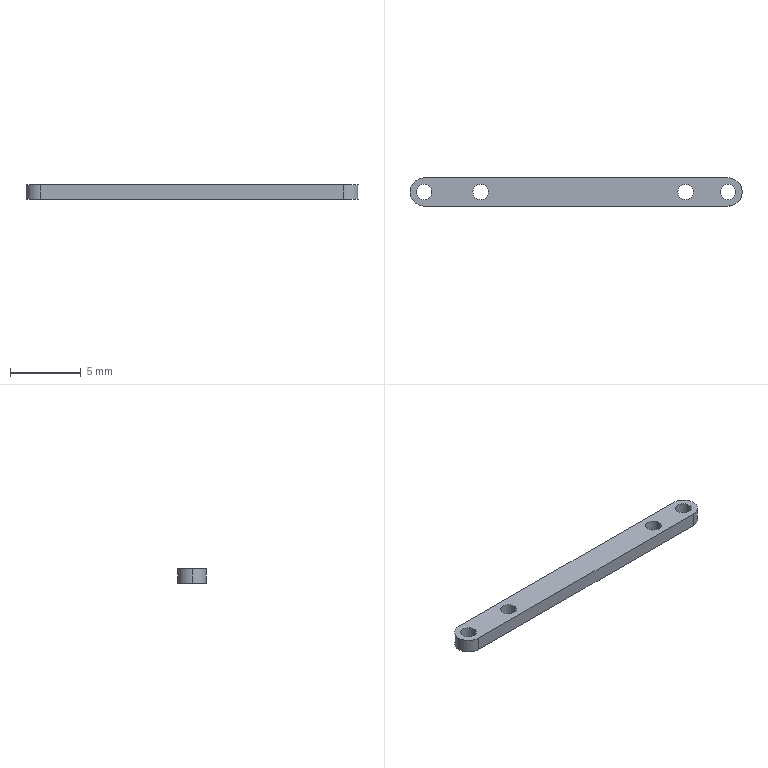Part | SolidWorks | features Extrusion 1, ICE 1 | 1 solid | 15 faces | box 23.5 x 2 x 1 mm | volume 42.34 mm3 | cylinder 11 | plane 4 | commonest cylinder face diameters 1.1 x8 2 x3
STEP:
#1=CARTESIAN_POINT('',(7.2,0.,0.5));
#2=VERTEX_POINT('',#1);
#3=CARTESIAN_POINT('',(8.3,0.,0.5));
#4=VERTEX_POINT('',#3);
#5=CARTESIAN_POINT('',(7.75,0.,0.5));
#6=DIRECTION('',(0.,0.,1.));
#7=DIRECTION('',(1.,0.,0.));
#8=AXIS2_PLACEMENT_3D('',#5,#6,#7);
#9=CIRCLE('',#8,0.55);
#10=EDGE_CURVE('',#2,#4,#9,.T.);
#11=ORIENTED_EDGE('',*,*,#10,.T.);
#12=CARTESIAN_POINT('',(8.3,0.,-0.5));
#13=VERTEX_POINT('',#12);
#14=CARTESIAN_POINT('',(8.3,0.,0.5));
#15=DIRECTION('',(0.,0.,-1.));
#16=VECTOR('',#15,1000.);
#17=LINE('',#14,#16);
#18=EDGE_CURVE('',#4,#13,#17,.T.);
#19=ORIENTED_EDGE('',*,*,#18,.T.);
#20=CARTESIAN_POINT('',(7.2,0.,-0.5));
#21=VERTEX_POINT('',#20);
#22=CARTESIAN_POINT('',(7.75,0.,-0.5));
#23=DIRECTION('',(0.,0.,1.));
#24=DIRECTION('',(1.,0.,0.));
#25=AXIS2_PLACEMENT_3D('',#22,#23,#24);
#26=CIRCLE('',#25,0.55);
#27=EDGE_CURVE('',#21,#13,#26,.T.);
#28=ORIENTED_EDGE('',*,*,#27,.F.);
#29=CARTESIAN_POINT('',(7.2,0.,0.5));
#30=DIRECTION('',(0.,0.,-1.));
#31=VECTOR('',#30,1000.);
#32=LINE('',#29,#31);
#33=EDGE_CURVE('',#2,#21,#32,.T.);
#34=ORIENTED_EDGE('',*,*,#33,.F.);
#35=EDGE_LOOP('',(#11,#19,#28,#34));
#36=FACE_OUTER_BOUND('',#35,.T.);
#37=CARTESIAN_POINT('',(7.75,0.,0.5));
#38=DIRECTION('',(0.,0.,-1.));
#39=DIRECTION('',(-1.,0.,0.));
#40=AXIS2_PLACEMENT_3D('',#37,#38,#39);
#41=CYLINDRICAL_SURFACE('',#40,0.55);
#42=ADVANCED_FACE('',(#36),#41,.F.);
#43=CARTESIAN_POINT('',(-7.3,0.,0.5));
#44=VERTEX_POINT('',#43);
#45=CARTESIAN_POINT('',(-6.2,0.,0.5));
#46=VERTEX_POINT('',#45);
#47=CARTESIAN_POINT('',(-6.75,0.,0.5));
#48=DIRECTION('',(0.,0.,1.));
#49=DIRECTION('',(1.,0.,0.));
#50=AXIS2_PLACEMENT_3D('',#47,#48,#49);
#51=CIRCLE('',#50,0.55);
#52=EDGE_CURVE('',#44,#46,#51,.T.);
#53=ORIENTED_EDGE('',*,*,#52,.T.);
#54=CARTESIAN_POINT('',(-6.2,0.,-0.5));
#55=VERTEX_POINT('',#54);
#56=CARTESIAN_POINT('',(-6.2,0.,0.5));
#57=DIRECTION('',(0.,0.,-1.));
#58=VECTOR('',#57,1000.);
#59=LINE('',#56,#58);
#60=EDGE_CURVE('',#46,#55,#59,.T.);
#61=ORIENTED_EDGE('',*,*,#60,.T.);
#62=CARTESIAN_POINT('',(-7.3,0.,-0.5));
#63=VERTEX_POINT('',#62);
#64=CARTESIAN_POINT('',(-6.75,0.,-0.5));
#65=DIRECTION('',(0.,0.,1.));
#66=DIRECTION('',(1.,0.,0.));
#67=AXIS2_PLACEMENT_3D('',#64,#65,#66);
#68=CIRCLE('',#67,0.55);
#69=EDGE_CURVE('',#63,#55,#68,.T.);
#70=ORIENTED_EDGE('',*,*,#69,.F.);
#71=CARTESIAN_POINT('',(-7.3,0.,0.5));
#72=DIRECTION('',(0.,0.,-1.));
#73=VECTOR('',#72,1000.);
#74=LINE('',#71,#73);
#75=EDGE_CURVE('',#44,#63,#74,.T.);
#76=ORIENTED_EDGE('',*,*,#75,.F.);
#77=EDGE_LOOP('',(#53,#61,#70,#76));
#78=FACE_OUTER_BOUND('',#77,.T.);
#79=CARTESIAN_POINT('',(-6.75,0.,0.5));
#80=DIRECTION('',(0.,0.,-1.));
#81=DIRECTION('',(-1.,0.,0.));
#82=AXIS2_PLACEMENT_3D('',#79,#80,#81);
#83=CYLINDRICAL_SURFACE('',#82,0.55);
#84=ADVANCED_FACE('',(#78),#83,.F.);
#85=CARTESIAN_POINT('',(10.2,0.,0.5));
#86=VERTEX_POINT('',#85);
#87=CARTESIAN_POINT('',(11.3,0.,0.5));
#88=VERTEX_POINT('',#87);
#89=CARTESIAN_POINT('',(10.75,0.,0.5));
#90=DIRECTION('',(0.,0.,1.));
#91=DIRECTION('',(1.,0.,0.));
#92=AXIS2_PLACEMENT_3D('',#89,#90,#91);
#93=CIRCLE('',#92,0.55);
#94=EDGE_CURVE('',#86,#88,#93,.T.);
#95=ORIENTED_EDGE('',*,*,#94,.T.);
#96=CARTESIAN_POINT('',(11.3,0.,-0.5));
#97=VERTEX_POINT('',#96);
#98=CARTESIAN_POINT('',(11.3,0.,0.5));
#99=DIRECTION('',(0.,0.,-1.));
#100=VECTOR('',#99,1000.);
#101=LINE('',#98,#100);
#102=EDGE_CURVE('',#88,#97,#101,.T.);
#103=ORIENTED_EDGE('',*,*,#102,.T.);
#104=CARTESIAN_POINT('',(10.2,0.,-0.5));
#105=VERTEX_POINT('',#104);
#106=CARTESIAN_POINT('',(10.75,0.,-0.5));
#107=DIRECTION('',(0.,0.,1.));
#108=DIRECTION('',(1.,0.,0.));
#109=AXIS2_PLACEMENT_3D('',#106,#107,#108);
#110=CIRCLE('',#109,0.55);
#111=EDGE_CURVE('',#105,#97,#110,.T.);
#112=ORIENTED_EDGE('',*,*,#111,.F.);
#113=CARTESIAN_POINT('',(10.2,0.,0.5));
#114=DIRECTION('',(0.,0.,-1.));
#115=VECTOR('',#114,1000.);
#116=LINE('',#113,#115);
#117=EDGE_CURVE('',#86,#105,#116,.T.);
#118=ORIENTED_EDGE('',*,*,#117,.F.);
#119=EDGE_LOOP('',(#95,#103,#112,#118));
#120=FACE_OUTER_BOUND('',#119,.T.);
#121=CARTESIAN_POINT('',(10.75,0.,0.5));
#122=DIRECTION('',(0.,0.,-1.));
#123=DIRECTION('',(-1.,0.,0.));
#124=AXIS2_PLACEMENT_3D('',#121,#122,#123);
#125=CYLINDRICAL_SURFACE('',#124,0.55);
#126=ADVANCED_FACE('',(#120),#125,.F.);
#127=CARTESIAN_POINT('',(-11.3,0.,0.5));
#128=VERTEX_POINT('',#127);
#129=CARTESIAN_POINT('',(-10.2,0.,0.5));
#130=VERTEX_POINT('',#129);
#131=CARTESIAN_POINT('',(-10.75,0.,0.5));
#132=DIRECTION('',(0.,0.,1.));
#133=DIRECTION('',(1.,0.,0.));
#134=AXIS2_PLACEMENT_3D('',#131,#132,#133);
#135=CIRCLE('',#134,0.55);
#136=EDGE_CURVE('',#128,#130,#135,.T.);
#137=ORIENTED_EDGE('',*,*,#136,.T.);
#138=CARTESIAN_POINT('',(-10.2,0.,-0.5));
#139=VERTEX_POINT('',#138);
#140=CARTESIAN_POINT('',(-10.2,0.,0.5));
#141=DIRECTION('',(0.,0.,-1.));
#142=VECTOR('',#141,1000.);
#143=LINE('',#140,#142);
#144=EDGE_CURVE('',#130,#139,#143,.T.);
#145=ORIENTED_EDGE('',*,*,#144,.T.);
#146=CARTESIAN_POINT('',(-11.3,0.,-0.5));
#147=VERTEX_POINT('',#146);
#148=CARTESIAN_POINT('',(-10.75,0.,-0.5));
#149=DIRECTION('',(0.,0.,1.));
#150=DIRECTION('',(1.,0.,0.));
#151=AXIS2_PLACEMENT_3D('',#148,#149,#150);
#152=CIRCLE('',#151,0.55);
#153=EDGE_CURVE('',#147,#139,#152,.T.);
#154=ORIENTED_EDGE('',*,*,#153,.F.);
#155=CARTESIAN_POINT('',(-11.3,0.,0.5));
#156=DIRECTION('',(0.,0.,-1.));
#157=VECTOR('',#156,1000.);
#158=LINE('',#155,#157);
#159=EDGE_CURVE('',#128,#147,#158,.T.);
#160=ORIENTED_EDGE('',*,*,#159,.F.);
#161=EDGE_LOOP('',(#137,#145,#154,#160));
#162=FACE_OUTER_BOUND('',#161,.T.);
#163=CARTESIAN_POINT('',(-10.75,0.,0.5));
#164=DIRECTION('',(0.,0.,-1.));
#165=DIRECTION('',(-1.,0.,0.));
#166=AXIS2_PLACEMENT_3D('',#163,#164,#165);
#167=CYLINDRICAL_SURFACE('',#166,0.55);
#168=ADVANCED_FACE('',(#162),#167,.F.);
#169=CARTESIAN_POINT('',(-11.75,0.,0.5));
#170=VERTEX_POINT('',#169);
#171=CARTESIAN_POINT('',(-10.75,-1.,0.5));
#172=VERTEX_POINT('',#171);
#173=CARTESIAN_POINT('',(-10.75,0.,0.5));
#174=DIRECTION('',(0.,0.,1.));
#175=DIRECTION('',(1.,0.,0.));
#176=AXIS2_PLACEMENT_3D('',#173,#174,#175);
#177=CIRCLE('',#176,1.);
#178=EDGE_CURVE('',#170,#172,#177,.T.);
#179=ORIENTED_EDGE('',*,*,#178,.F.);
#180=CARTESIAN_POINT('',(-11.75,0.,-0.5));
#181=VERTEX_POINT('',#180);
#182=CARTESIAN_POINT('',(-11.75,0.,0.5));
#183=DIRECTION('',(0.,0.,-1.));
#184=VECTOR('',#183,1000.);
#185=LINE('',#182,#184);
#186=EDGE_CURVE('',#170,#181,#185,.T.);
#187=ORIENTED_EDGE('',*,*,#186,.T.);
#188=CARTESIAN_POINT('',(-10.75,-1.,-0.5));
#189=VERTEX_POINT('',#188);
#190=CARTESIAN_POINT('',(-10.75,0.,-0.5));
#191=DIRECTION('',(0.,0.,1.));
#192=DIRECTION('',(1.,0.,0.));
#193=AXIS2_PLACEMENT_3D('',#190,#191,#192);
#194=CIRCLE('',#193,1.);
#195=EDGE_CURVE('',#181,#189,#194,.T.);
#196=ORIENTED_EDGE('',*,*,#195,.T.);
#197=CARTESIAN_POINT('',(-10.75,-1.,0.5));
#198=DIRECTION('',(0.,0.,-1.));
#199=VECTOR('',#198,1000.);
#200=LINE('',#197,#199);
#201=EDGE_CURVE('',#172,#189,#200,.T.);
#202=ORIENTED_EDGE('',*,*,#201,.F.);
#203=EDGE_LOOP('',(#179,#187,#196,#202));
#204=FACE_OUTER_BOUND('',#203,.T.);
#205=CARTESIAN_POINT('',(-10.75,0.,0.5));
#206=DIRECTION('',(0.,0.,-1.));
#207=DIRECTION('',(-1.,0.,0.));
#208=AXIS2_PLACEMENT_3D('',#205,#206,#207);
#209=CYLINDRICAL_SURFACE('',#208,1.);
#210=ADVANCED_FACE('',(#204),#209,.T.);
#211=ORIENTED_EDGE('',*,*,#52,.F.);
#212=CARTESIAN_POINT('',(-6.75,0.,0.5));
#213=DIRECTION('',(0.,0.,1.));
#214=DIRECTION('',(1.,0.,0.));
#215=AXIS2_PLACEMENT_3D('',#212,#213,#214);
#216=CIRCLE('',#215,0.55);
#217=EDGE_CURVE('',#46,#44,#216,.T.);
#218=ORIENTED_EDGE('',*,*,#217,.F.);
#219=EDGE_LOOP('',(#211,#218));
#220=FACE_BOUND('',#219,.T.);
#221=ORIENTED_EDGE('',*,*,#136,.F.);
#222=CARTESIAN_POINT('',(-10.75,0.,0.5));
#223=DIRECTION('',(0.,0.,1.));
#224=DIRECTION('',(1.,0.,0.));
#225=AXIS2_PLACEMENT_3D('',#222,#223,#224);
#226=CIRCLE('',#225,0.55);
#227=EDGE_CURVE('',#130,#128,#226,.T.);
#228=ORIENTED_EDGE('',*,*,#227,.F.);
#229=EDGE_LOOP('',(#221,#228));
#230=FACE_BOUND('',#229,.T.);
#231=CARTESIAN_POINT('',(-10.75,1.,0.5));
#232=VERTEX_POINT('',#231);
#233=CARTESIAN_POINT('',(-10.75,0.,0.5));
#234=DIRECTION('',(0.,0.,1.));
#235=DIRECTION('',(1.,0.,0.));
#236=AXIS2_PLACEMENT_3D('',#233,#234,#235);
#237=CIRCLE('',#236,1.);
#238=EDGE_CURVE('',#232,#170,#237,.T.);
#239=ORIENTED_EDGE('',*,*,#238,.T.);
#240=ORIENTED_EDGE('',*,*,#178,.T.);
#241=CARTESIAN_POINT('',(10.75,-1.,0.5));
#242=VERTEX_POINT('',#241);
#243=CARTESIAN_POINT('',(-10.75,-1.,0.5));
#244=DIRECTION('',(1.,0.,0.));
#245=VECTOR('',#244,1000.);
#246=LINE('',#243,#245);
#247=EDGE_CURVE('',#172,#242,#246,.T.);
#248=ORIENTED_EDGE('',*,*,#247,.T.);
#249=CARTESIAN_POINT('',(10.75,1.,0.5));
#250=VERTEX_POINT('',#249);
#251=CARTESIAN_POINT('',(10.75,0.,0.5));
#252=DIRECTION('',(0.,0.,1.));
#253=DIRECTION('',(1.,0.,0.));
#254=AXIS2_PLACEMENT_3D('',#251,#252,#253);
#255=CIRCLE('',#254,1.);
#256=EDGE_CURVE('',#242,#250,#255,.T.);
#257=ORIENTED_EDGE('',*,*,#256,.T.);
#258=CARTESIAN_POINT('',(-10.75,1.,0.5));
#259=DIRECTION('',(-1.,0.,0.));
#260=VECTOR('',#259,1000.);
#261=LINE('',#258,#260);
#262=EDGE_CURVE('',#250,#232,#261,.T.);
#263=ORIENTED_EDGE('',*,*,#262,.T.);
#264=EDGE_LOOP('',(#239,#240,#248,#257,#263));
#265=FACE_OUTER_BOUND('',#264,.T.);
#266=ORIENTED_EDGE('',*,*,#94,.F.);
#267=CARTESIAN_POINT('',(10.75,0.,0.5));
#268=DIRECTION('',(0.,0.,1.));
#269=DIRECTION('',(1.,0.,0.));
#270=AXIS2_PLACEMENT_3D('',#267,#268,#269);
#271=CIRCLE('',#270,0.55);
#272=EDGE_CURVE('',#88,#86,#271,.T.);
#273=ORIENTED_EDGE('',*,*,#272,.F.);
#274=EDGE_LOOP('',(#266,#273));
#275=FACE_BOUND('',#274,.T.);
#276=ORIENTED_EDGE('',*,*,#10,.F.);
#277=CARTESIAN_POINT('',(7.75,0.,0.5));
#278=DIRECTION('',(0.,0.,1.));
#279=DIRECTION('',(1.,0.,0.));
#280=AXIS2_PLACEMENT_3D('',#277,#278,#279);
#281=CIRCLE('',#280,0.55);
#282=EDGE_CURVE('',#4,#2,#281,.T.);
#283=ORIENTED_EDGE('',*,*,#282,.F.);
#284=EDGE_LOOP('',(#276,#283));
#285=FACE_BOUND('',#284,.T.);
#286=CARTESIAN_POINT('',(-10.75,0.,0.5));
#287=DIRECTION('',(0.,0.,1.));
#288=DIRECTION('',(1.,0.,0.));
#289=AXIS2_PLACEMENT_3D('',#286,#287,#288);
#290=PLANE('',#289);
#291=ADVANCED_FACE('',(#220,#230,#265,#275,#285),#290,.T.);
#292=CARTESIAN_POINT('',(-10.75,1.,-0.5));
#293=VERTEX_POINT('',#292);
#294=CARTESIAN_POINT('',(-10.75,0.,-0.5));
#295=DIRECTION('',(0.,0.,1.));
#296=DIRECTION('',(1.,0.,0.));
#297=AXIS2_PLACEMENT_3D('',#294,#295,#296);
#298=CIRCLE('',#297,1.);
#299=EDGE_CURVE('',#293,#181,#298,.T.);
#300=ORIENTED_EDGE('',*,*,#299,.F.);
#301=CARTESIAN_POINT('',(10.75,1.,-0.5));
#302=VERTEX_POINT('',#301);
#303=CARTESIAN_POINT('',(-10.75,1.,-0.5));
#304=DIRECTION('',(-1.,0.,0.));
#305=VECTOR('',#304,1000.);
#306=LINE('',#303,#305);
#307=EDGE_CURVE('',#302,#293,#306,.T.);
#308=ORIENTED_EDGE('',*,*,#307,.F.);
#309=CARTESIAN_POINT('',(10.75,-1.,-0.5));
#310=VERTEX_POINT('',#309);
#311=CARTESIAN_POINT('',(10.75,0.,-0.5));
#312=DIRECTION('',(0.,0.,1.));
#313=DIRECTION('',(1.,0.,0.));
#314=AXIS2_PLACEMENT_3D('',#311,#312,#313);
#315=CIRCLE('',#314,1.);
#316=EDGE_CURVE('',#310,#302,#315,.T.);
#317=ORIENTED_EDGE('',*,*,#316,.F.);
#318=CARTESIAN_POINT('',(-10.75,-1.,-0.5));
#319=DIRECTION('',(1.,0.,0.));
#320=VECTOR('',#319,1000.);
#321=LINE('',#318,#320);
#322=EDGE_CURVE('',#189,#310,#321,.T.);
#323=ORIENTED_EDGE('',*,*,#322,.F.);
#324=ORIENTED_EDGE('',*,*,#195,.F.);
#325=EDGE_LOOP('',(#300,#308,#317,#323,#324));
#326=FACE_OUTER_BOUND('',#325,.T.);
#327=ORIENTED_EDGE('',*,*,#153,.T.);
#328=CARTESIAN_POINT('',(-10.75,0.,-0.5));
#329=DIRECTION('',(0.,0.,1.));
#330=DIRECTION('',(1.,0.,0.));
#331=AXIS2_PLACEMENT_3D('',#328,#329,#330);
#332=CIRCLE('',#331,0.55);
#333=EDGE_CURVE('',#139,#147,#332,.T.);
#334=ORIENTED_EDGE('',*,*,#333,.T.);
#335=EDGE_LOOP('',(#327,#334));
#336=FACE_BOUND('',#335,.T.);
#337=ORIENTED_EDGE('',*,*,#111,.T.);
#338=CARTESIAN_POINT('',(10.75,0.,-0.5));
#339=DIRECTION('',(0.,0.,1.));
#340=DIRECTION('',(1.,0.,0.));
#341=AXIS2_PLACEMENT_3D('',#338,#339,#340);
#342=CIRCLE('',#341,0.55);
#343=EDGE_CURVE('',#97,#105,#342,.T.);
#344=ORIENTED_EDGE('',*,*,#343,.T.);
#345=EDGE_LOOP('',(#337,#344));
#346=FACE_BOUND('',#345,.T.);
#347=ORIENTED_EDGE('',*,*,#69,.T.);
#348=CARTESIAN_POINT('',(-6.75,0.,-0.5));
#349=DIRECTION('',(0.,0.,1.));
#350=DIRECTION('',(1.,0.,0.));
#351=AXIS2_PLACEMENT_3D('',#348,#349,#350);
#352=CIRCLE('',#351,0.55);
#353=EDGE_CURVE('',#55,#63,#352,.T.);
#354=ORIENTED_EDGE('',*,*,#353,.T.);
#355=EDGE_LOOP('',(#347,#354));
#356=FACE_BOUND('',#355,.T.);
#357=ORIENTED_EDGE('',*,*,#27,.T.);
#358=CARTESIAN_POINT('',(7.75,0.,-0.5));
#359=DIRECTION('',(0.,0.,1.));
#360=DIRECTION('',(1.,0.,0.));
#361=AXIS2_PLACEMENT_3D('',#358,#359,#360);
#362=CIRCLE('',#361,0.55);
#363=EDGE_CURVE('',#13,#21,#362,.T.);
#364=ORIENTED_EDGE('',*,*,#363,.T.);
#365=EDGE_LOOP('',(#357,#364));
#366=FACE_BOUND('',#365,.T.);
#367=CARTESIAN_POINT('',(-10.75,0.,-0.5));
#368=DIRECTION('',(0.,0.,1.));
#369=DIRECTION('',(1.,0.,0.));
#370=AXIS2_PLACEMENT_3D('',#367,#368,#369);
#371=PLANE('',#370);
#372=ADVANCED_FACE('',(#326,#336,#346,#356,#366),#371,.F.);
#373=ORIENTED_EDGE('',*,*,#186,.F.);
#374=ORIENTED_EDGE('',*,*,#238,.F.);
#375=CARTESIAN_POINT('',(-10.75,1.,0.5));
#376=DIRECTION('',(0.,0.,-1.));
#377=VECTOR('',#376,1000.);
#378=LINE('',#375,#377);
#379=EDGE_CURVE('',#232,#293,#378,.T.);
#380=ORIENTED_EDGE('',*,*,#379,.T.);
#381=ORIENTED_EDGE('',*,*,#299,.T.);
#382=EDGE_LOOP('',(#373,#374,#380,#381));
#383=FACE_OUTER_BOUND('',#382,.T.);
#384=CARTESIAN_POINT('',(-10.75,0.,0.5));
#385=DIRECTION('',(0.,0.,-1.));
#386=DIRECTION('',(-1.,0.,0.));
#387=AXIS2_PLACEMENT_3D('',#384,#385,#386);
#388=CYLINDRICAL_SURFACE('',#387,1.);
#389=ADVANCED_FACE('',(#383),#388,.T.);
#390=ORIENTED_EDGE('',*,*,#322,.T.);
#391=CARTESIAN_POINT('',(10.75,-1.,0.5));
#392=DIRECTION('',(0.,0.,-1.));
#393=VECTOR('',#392,1000.);
#394=LINE('',#391,#393);
#395=EDGE_CURVE('',#242,#310,#394,.T.);
#396=ORIENTED_EDGE('',*,*,#395,.F.);
#397=ORIENTED_EDGE('',*,*,#247,.F.);
#398=ORIENTED_EDGE('',*,*,#201,.T.);
#399=EDGE_LOOP('',(#390,#396,#397,#398));
#400=FACE_OUTER_BOUND('',#399,.T.);
#401=CARTESIAN_POINT('',(-10.75,-1.,0.5));
#402=DIRECTION('',(0.,1.,0.));
#403=DIRECTION('',(-1.,0.,0.));
#404=AXIS2_PLACEMENT_3D('',#401,#402,#403);
#405=PLANE('',#404);
#406=ADVANCED_FACE('',(#400),#405,.F.);
#407=ORIENTED_EDGE('',*,*,#316,.T.);
#408=CARTESIAN_POINT('',(10.75,1.,0.5));
#409=DIRECTION('',(0.,0.,-1.));
#410=VECTOR('',#409,1000.);
#411=LINE('',#408,#410);
#412=EDGE_CURVE('',#250,#302,#411,.T.);
#413=ORIENTED_EDGE('',*,*,#412,.F.);
#414=ORIENTED_EDGE('',*,*,#256,.F.);
#415=ORIENTED_EDGE('',*,*,#395,.T.);
#416=EDGE_LOOP('',(#407,#413,#414,#415));
#417=FACE_OUTER_BOUND('',#416,.T.);
#418=CARTESIAN_POINT('',(10.75,0.,0.5));
#419=DIRECTION('',(0.,0.,-1.));
#420=DIRECTION('',(-1.,0.,0.));
#421=AXIS2_PLACEMENT_3D('',#418,#419,#420);
#422=CYLINDRICAL_SURFACE('',#421,1.);
#423=ADVANCED_FACE('',(#417),#422,.T.);
#424=ORIENTED_EDGE('',*,*,#307,.T.);
#425=ORIENTED_EDGE('',*,*,#379,.F.);
#426=ORIENTED_EDGE('',*,*,#262,.F.);
#427=ORIENTED_EDGE('',*,*,#412,.T.);
#428=EDGE_LOOP('',(#424,#425,#426,#427));
#429=FACE_OUTER_BOUND('',#428,.T.);
#430=CARTESIAN_POINT('',(-10.75,1.,0.5));
#431=DIRECTION('',(0.,-1.,0.));
#432=DIRECTION('',(1.,0.,0.));
#433=AXIS2_PLACEMENT_3D('',#430,#431,#432);
#434=PLANE('',#433);
#435=ADVANCED_FACE('',(#429),#434,.F.);
#436=ORIENTED_EDGE('',*,*,#144,.F.);
#437=ORIENTED_EDGE('',*,*,#227,.T.);
#438=ORIENTED_EDGE('',*,*,#159,.T.);
#439=ORIENTED_EDGE('',*,*,#333,.F.);
#440=EDGE_LOOP('',(#436,#437,#438,#439));
#441=FACE_OUTER_BOUND('',#440,.T.);
#442=CARTESIAN_POINT('',(-10.75,0.,0.5));
#443=DIRECTION('',(0.,0.,-1.));
#444=DIRECTION('',(-1.,0.,0.));
#445=AXIS2_PLACEMENT_3D('',#442,#443,#444);
#446=CYLINDRICAL_SURFACE('',#445,0.55);
#447=ADVANCED_FACE('',(#441),#446,.F.);
#448=ORIENTED_EDGE('',*,*,#102,.F.);
#449=ORIENTED_EDGE('',*,*,#272,.T.);
#450=ORIENTED_EDGE('',*,*,#117,.T.);
#451=ORIENTED_EDGE('',*,*,#343,.F.);
#452=EDGE_LOOP('',(#448,#449,#450,#451));
#453=FACE_OUTER_BOUND('',#452,.T.);
#454=CARTESIAN_POINT('',(10.75,0.,0.5));
#455=DIRECTION('',(0.,0.,-1.));
#456=DIRECTION('',(-1.,0.,0.));
#457=AXIS2_PLACEMENT_3D('',#454,#455,#456);
#458=CYLINDRICAL_SURFACE('',#457,0.55);
#459=ADVANCED_FACE('',(#453),#458,.F.);
#460=ORIENTED_EDGE('',*,*,#60,.F.);
#461=ORIENTED_EDGE('',*,*,#217,.T.);
#462=ORIENTED_EDGE('',*,*,#75,.T.);
#463=ORIENTED_EDGE('',*,*,#353,.F.);
#464=EDGE_LOOP('',(#460,#461,#462,#463));
#465=FACE_OUTER_BOUND('',#464,.T.);
#466=CARTESIAN_POINT('',(-6.75,0.,0.5));
#467=DIRECTION('',(0.,0.,-1.));
#468=DIRECTION('',(-1.,0.,0.));
#469=AXIS2_PLACEMENT_3D('',#466,#467,#468);
#470=CYLINDRICAL_SURFACE('',#469,0.55);
#471=ADVANCED_FACE('',(#465),#470,.F.);
#472=ORIENTED_EDGE('',*,*,#18,.F.);
#473=ORIENTED_EDGE('',*,*,#282,.T.);
#474=ORIENTED_EDGE('',*,*,#33,.T.);
#475=ORIENTED_EDGE('',*,*,#363,.F.);
#476=EDGE_LOOP('',(#472,#473,#474,#475));
#477=FACE_OUTER_BOUND('',#476,.T.);
#478=CARTESIAN_POINT('',(7.75,0.,0.5));
#479=DIRECTION('',(0.,0.,-1.));
#480=DIRECTION('',(-1.,0.,0.));
#481=AXIS2_PLACEMENT_3D('',#478,#479,#480);
#482=CYLINDRICAL_SURFACE('',#481,0.55);
#483=ADVANCED_FACE('',(#477),#482,.F.);
#484=CLOSED_SHELL('',(#42,#84,#126,#168,#210,#291,#372,#389,#406,#423,#435,#447,#459,#471,#483));
#485=MANIFOLD_SOLID_BREP('',#484);
#486=CARTESIAN_POINT('',(0.,0.,0.));
#487=DIRECTION('',(0.,0.,1.));
#488=DIRECTION('',(1.,0.,0.));
#489=AXIS2_PLACEMENT_3D('',#486,#487,#488);
#490=(LENGTH_UNIT()NAMED_UNIT(*)SI_UNIT(.MILLI.,.METRE.));
#491=UNCERTAINTY_MEASURE_WITH_UNIT(LENGTH_MEASURE(0.00001),#490,'','');
#492=(NAMED_UNIT(*)PLANE_ANGLE_UNIT()SI_UNIT($,.RADIAN.));
#493=(NAMED_UNIT(*)SI_UNIT($,.STERADIAN.)SOLID_ANGLE_UNIT());
#494=(GEOMETRIC_REPRESENTATION_CONTEXT(3)GLOBAL_UNCERTAINTY_ASSIGNED_CONTEXT((#491))GLOBAL_UNIT_ASSIGNED_CONTEXT((#490,#492,#493))REPRESENTATION_CONTEXT('',''));
#495=ADVANCED_BREP_SHAPE_REPRESENTATION('',(#485,#489),#494);